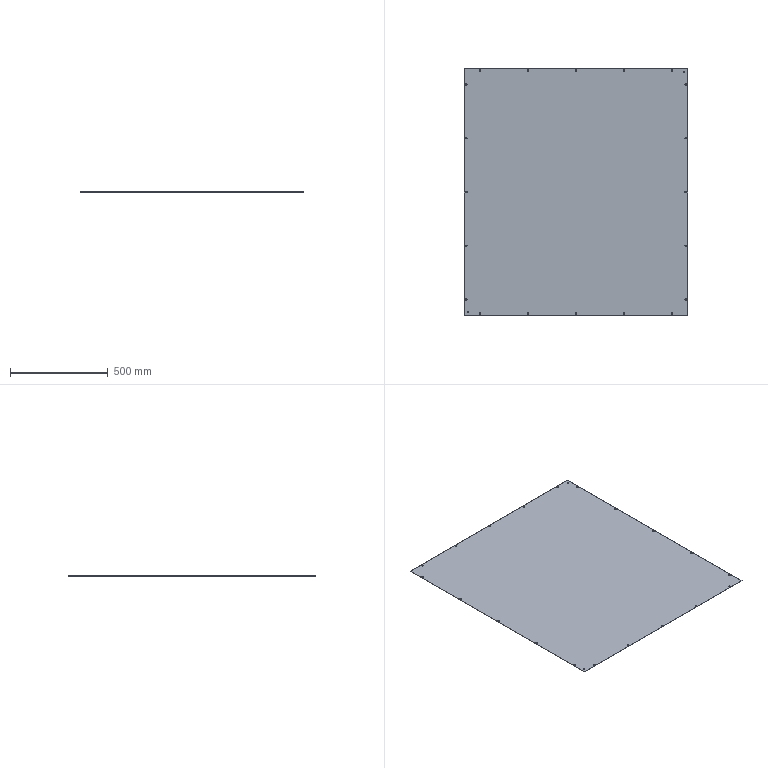Part | SolidWorks | features Cut 2, Extrusion 1 | 1 solid | 100 faces | box 1140 x 1260 x 1 mm | volume 1435171 mm3 | cylinder 54 | plane 46 | commonest cylinder face diameters 7 x50 5 x4